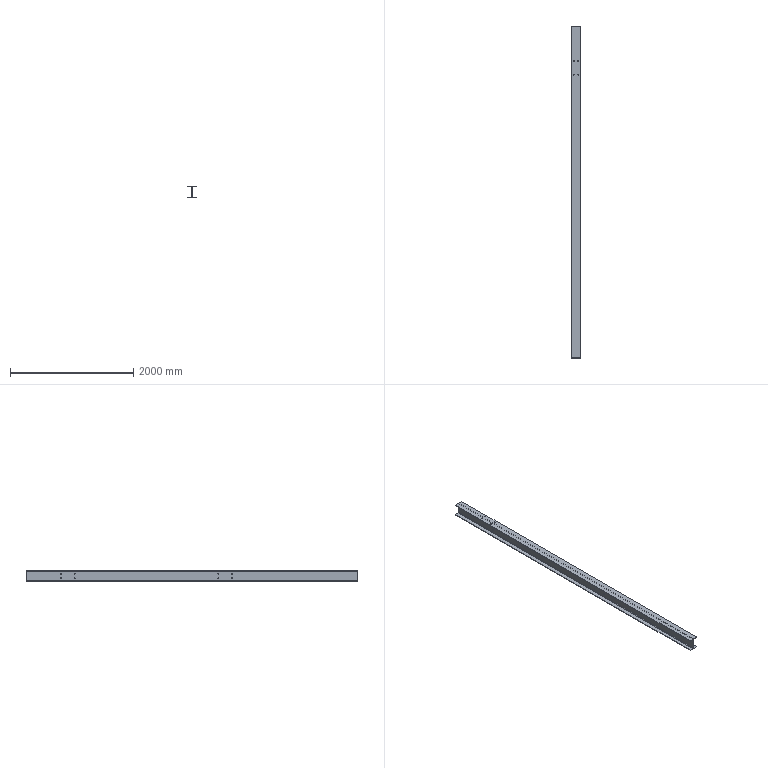Part | STEP file | 粉仓立柱2主体_Default<As Machined> | 1 solid | 42 faces | box 150 x 5378 x 194 mm | volume 20480381 mm3 | cylinder 28 | plane 14 | commonest cylinder face diameters 15 x24 16 x4